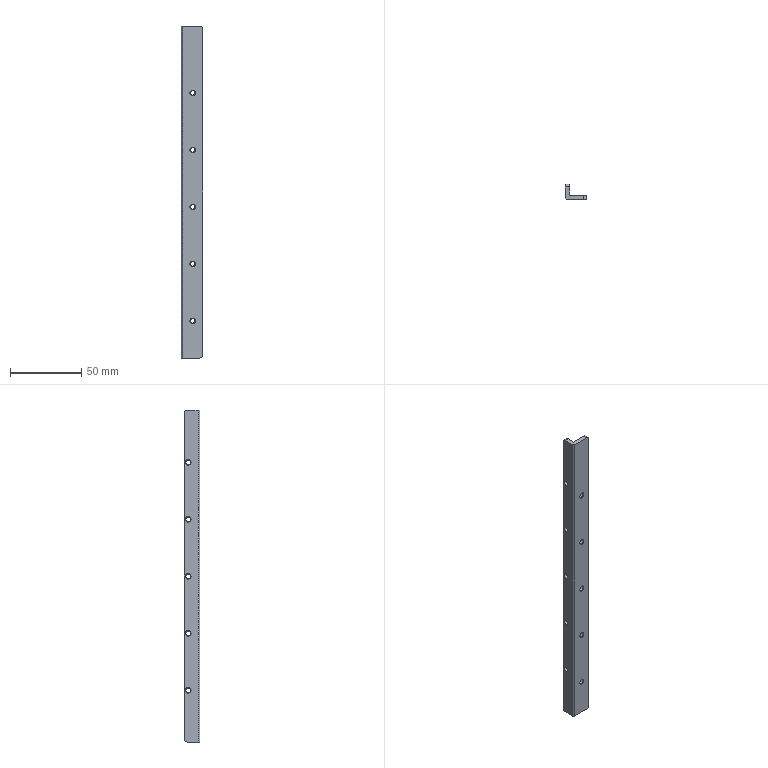Part | STEP file | L shaped aluminium angle 2 | 1 solid | 38 faces | box 15 x 10.7 x 233 mm | volume 15474 mm3 | cone 15 | cylinder 14 | plane 9 | commonest cylinder face diameters 3.3 x10 4 x4